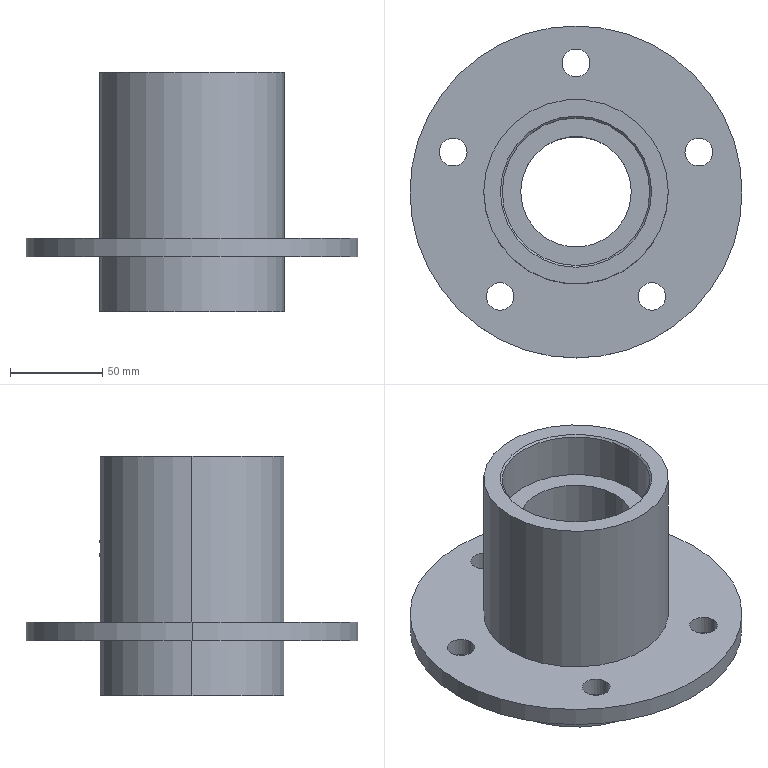Part | SolidWorks | features ICE 7, HoleWzd 2, Chamfer 1, Extrusion 1 | 2 solids | 68 faces | box 180 x 180 x 130 mm | volume 680348 mm3 | cylinder 42 | cone 18 | plane 8 | commonest cylinder face diameters 5 x14 15 x10 80 x6 100 x4 9 x2 60 x2